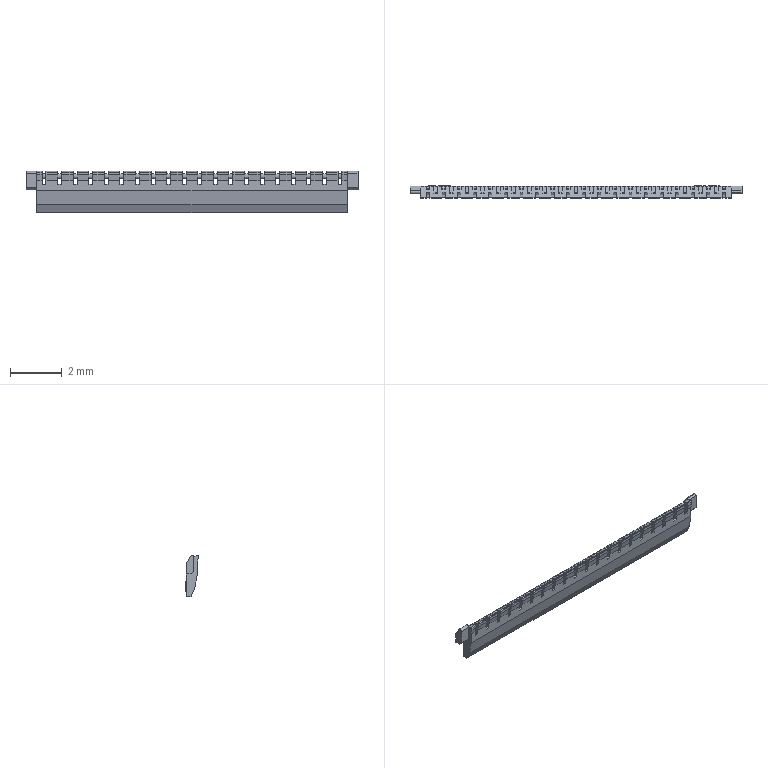Part | Creo | 1 solid | 437 faces | box 12.79 x 0.475 x 1.585 mm | volume 6 mm3 | plane 319 | cylinder 118 | commonest cylinder face diameters 0.06 x42 0.2 x40 0.4 x19 0.093 x14 0.14 x3